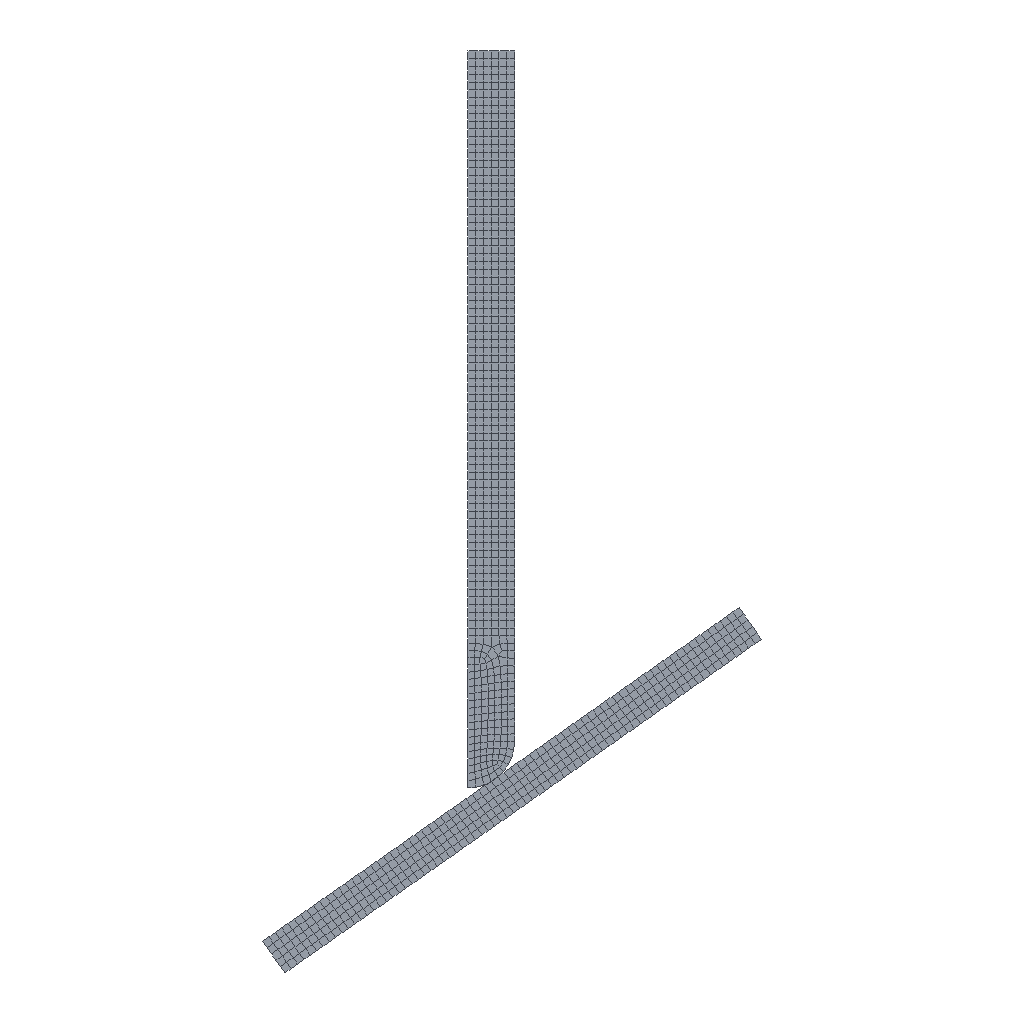Simulation study | abaqus
Set-up summary:
category,name,step,type,value,unit,region
solver,abaqus
solver,version,,,Abaqus/Standard 2020
units,not stated in the deck,,not stated
analysis,deck,,static,static
load_step,Step-1,Step-1,static
load_step,requested,,,1
mesh,nodes,,,1144
mesh,elements,,,962
element_type,CPS4R,,plane,962
load,load commands in deck,,count,1
bc,support commands in deck,,count,4
material,PIDAI,,in results
material,QUNBAN,,in results
check,setup vs results,,match,"per instance, exact: element labels, types and connectivity; labels of the nodes the elements use; coordinates of those nodes at SINGLE_PRECISION in 2 of 2 instance(s)"
Abaqus input file, long lists of numbers shortened:
*Heading
** Job name: Job-1 Model name: Model-1
** Generated by: Abaqus/CAE 2020
*Preprint, echo=NO, model=NO, history=NO, contact=NO
**
** PARTS
**
*Part, name=pidai
*Node
      1,         500.,         110.
      2,         500.,         108.
** (454 more lines like these left out)
*Element, type=CPS4R
  1,   1,   2,   8,   7
  2,   2,   3,   9,   8
** (373 more lines like these left out)
*Nset, nset=Set-1, generate
   1,  456,    1
*Elset, elset=Set-1, generate
   1,  375,    1
** Section: pidai
*Solid Section, elset=Set-1, material=pidai
,
*End Part
**
*Part, name=qunban
*Node
      1,   501.389,   174.615
      2,   513.389,   174.615
** (686 more lines like these left out)
*Element, type=CPS4R
  1,   1,   7, 206, 164
  2,   7,   8, 207, 206
** (585 more lines like these left out)
*Nset, nset=Set-1, generate
   1,  688,    1
*Elset, elset=Set-1, generate
   1,  587,    1
** Section: qunban
*Solid Section, elset=Set-1, material=qunban
,
*End Part
**
**
** ASSEMBLY
**
*Assembly, name=Assembly
**
*Instance, name=pidai-1, part=pidai
101.955, -280.992,           0.
101.955, -280.992,           0., 101.955, -280.992, 1., 35.
*End Instance
**
*Instance, name=qunban-1, part=qunban
*End Instance
**
*Node
      1,   507.389,   325.407,           0.
*Node
      2,   515.61,   130.73,           0.
*Nset, nset=Set-2, instance=pidai-1, generate
   6,  456,    6
*Elset, elset=Set-2, instance=pidai-1, generate
   5,  375,    5
*Nset, nset=Set-3
 1,
*Nset, nset=Set-4, instance=qunban-1
  3,  4, 86, 87, 88, 89, 90
*Elset, elset=Set-4, instance=qunban-1, generate
 445,  450,    1
*Nset, nset=Set-7, instance=pidai-1
   1,   2,   3,   4,   5,   6,  12,  18,  24,  30,  36,  42,  48,  54,  60,  66
  72,  78,  84,  90,  96, 102, 108, 114, 120, 126, 132, 138, 144, 150, 156, 162
** (4 more lines like these left out)
*Elset, elset=Set-7, instance=pidai-1
   1,   2,   3,   4,   5,  10,  15,  20,  25,  30,  35,  40,  45,  50,  55,  60
  65,  70,  75,  80,  85,  90,  95, 100, 105, 110, 115, 120, 125, 130, 135, 140
** (4 more lines like these left out)
*Nset, nset=Set-8, instance=qunban-1
   1,   2,   3,   4,   7,   8,   9,  10,  11,  12,  13,  14,  15,  16,  17,  18
  19,  20,  21,  22,  23,  24,  25,  26,  27,  28,  29,  30,  31,  32,  33,  34
** (32 more lines like these left out)
*Nset, nset=Set-8
 1,
*Elset, elset=Set-8, instance=qunban-1, generate
   1,  450,    1
*Nset, nset=b_Set-5, instance=pidai-1, generate
   1,  456,    1
*Elset, elset=b_Set-5, instance=pidai-1, generate
   1,  375,    1
*Nset, nset=m_Set-1
 1,
*Nset, nset=_PickedSet19, internal
 2,
*Elset, elset=_m_Surf-1_S2, internal, instance=qunban-1
 461, 482, 485, 499, 500, 501
*Elset, elset=_m_Surf-1_S4, internal, instance=qunban-1
 463, 483, 484
*Surface, type=ELEMENT, name=m_Surf-1
_m_Surf-1_S2, S2
_m_Surf-1_S4, S4
*Elset, elset=_m_Surf-4_S2, internal, instance=qunban-1
   6,  12,  18,  24,  30,  36,  42,  48,  54,  60,  66,  72,  78,  84,  90,  96
 102, 108, 114, 120, 126, 132, 138, 144, 150, 156, 162, 168, 174, 180, 186, 192
** (4 more lines like these left out)
*Elset, elset=_m_Surf-4_S4, internal, instance=qunban-1
 459, 463, 483, 484, 486, 510, 530
*Surface, type=ELEMENT, name=m_Surf-4
_m_Surf-4_S2, S2
_m_Surf-4_S4, S4
*Elset, elset=_m_Surf-6_S2, internal, instance=qunban-1
   6,  12,  18,  24,  30,  36,  42,  48,  54,  60,  66,  72,  78,  84,  90,  96
 102, 108, 114, 120, 126, 132, 138, 144, 150, 156, 162, 168, 174, 180, 186, 192
** (4 more lines like these left out)
*Elset, elset=_m_Surf-6_S4, internal, instance=qunban-1
   1,   7,  13,  19,  25,  31,  37,  43,  49,  55,  61,  67,  73,  79,  85,  91
  97, 103, 109, 115, 121, 127, 133, 139, 145, 151, 157, 163, 169, 175, 181, 187
** (4 more lines like these left out)
*Elset, elset=_m_Surf-6_S3, internal, instance=qunban-1
 453, 462, 465, 474, 475, 479, 480, 502, 503
*Elset, elset=_m_Surf-6_S1, internal, instance=qunban-1
 456, 457, 461, 467, 469, 470, 471, 472, 476, 477, 498, 515
*Surface, type=ELEMENT, name=m_Surf-6
_m_Surf-6_S2, S2
_m_Surf-6_S4, S4
_m_Surf-6_S3, S3
_m_Surf-6_S1, S1
*Elset, elset=_s_Surf-1_S4, internal, instance=pidai-1, generate
   1,  371,    5
*Surface, type=ELEMENT, name=s_Surf-1
_s_Surf-1_S4, S4
*Elset, elset=_s_Surf-3_S3, internal, instance=qunban-1, generate
 445,  450,    1
*Surface, type=ELEMENT, name=s_Surf-3
_s_Surf-3_S3, S3
*Elset, elset=_s_Surf-4_S4, internal, instance=pidai-1, generate
   1,  371,    5
*Surface, type=ELEMENT, name=s_Surf-4
_s_Surf-4_S4, S4
*End Assembly
*Amplitude, name=Amp-1
             0.,              1.,              1.,              1.
*Amplitude, name=Amp-2
             0.,              0.,              1.,              1.
**
** MATERIALS
**
*Material, name=pidai
*Density
 1.35e-09,
*Elastic
 0.1, 0.47
*Material, name=qunban
*Hyperelastic, mooney-rivlin
 0.483, 0.121,    0.
**
** INTERACTION PROPERTIES
**
*Surface Interaction, name=IntProp-1
1.,
*Friction, slip tolerance=0.005
 0.5,
*Surface Behavior, pressure-overclosure=HARD
**
** BOUNDARY CONDITIONS
**
** Name: BC-1 Type: 对称/反对称/完全固定
*Boundary
Set-7, ENCASTRE
**
** INTERACTIONS
**
** Interaction: Int-1
*Contact Pair, interaction=IntProp-1, type=SURFACE TO SURFACE
s_Surf-4, m_Surf-6
** ----------------------------------------------------------------
**
** STEP: Step-1
**
*Step, name=Step-1, nlgeom=YES, inc=1000
*Static, stabilize=0.0002, allsdtol=0.05, continue=NO
0.001, 1., 1e-05, 1.
**
** BOUNDARY CONDITIONS
**
** Name: BC-2 Type: 位移/转角
*Boundary, amplitude=Amp-2
Set-8, 1, 1
Set-8, 2, 2, -1.
Set-8, 6, 6
**
** OUTPUT REQUESTS
**
*Restart, write, frequency=0
**
** FIELD OUTPUT: F-Output-1
**
*Output, field
*Node Output
RF, RT, U, V
*Element Output, directions=YES
E, LE, MISES, MISESMAX, PE, PEEQ, PEMAG, S, SF
*Contact Output
CDISP, CSTRESS
*Output, history, frequency=0
*End Step
Results summary:
result,step,,completed,increments=17 time=1.0/1.0
result,analysis,,,static
result,last_loadstep,,,1
result,primary field,,,U
result,reaction total,,FX,-2e-06,model units
result,reaction total,,FY,-7.7e-05,model units
result,reaction total,,FZ,0.0,model units